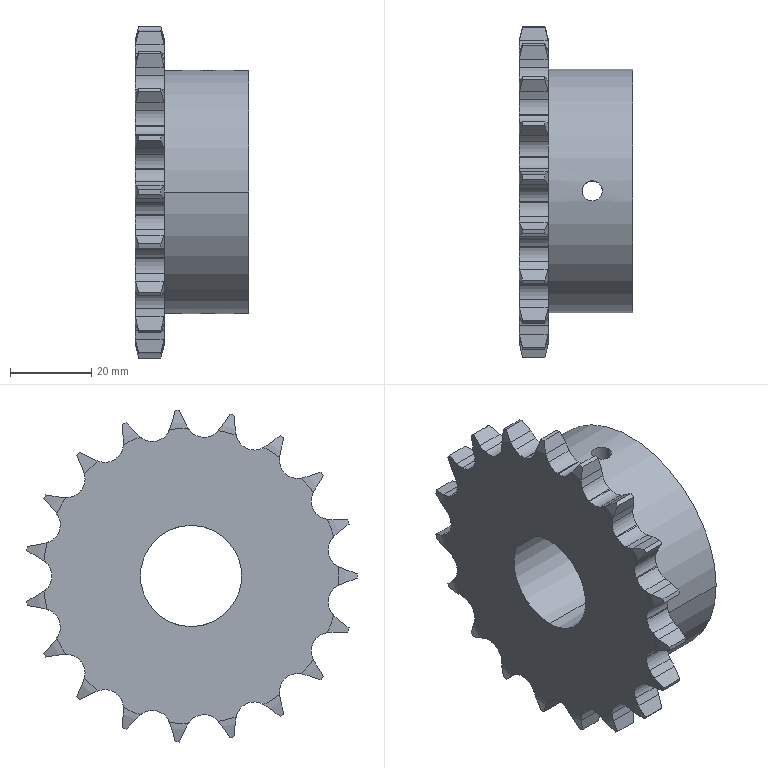Part | STEP file | 2108-191V11 | 1 solid | 201 faces | box 28 x 81.525 x 81.8 mm | volume 74497 mm3 | cylinder 103 | plane 60 | torus 38 | commonest cylinder face diameters 8.561 x38 22.126 x38 82 x19 5 x4 25 x2 60 x2